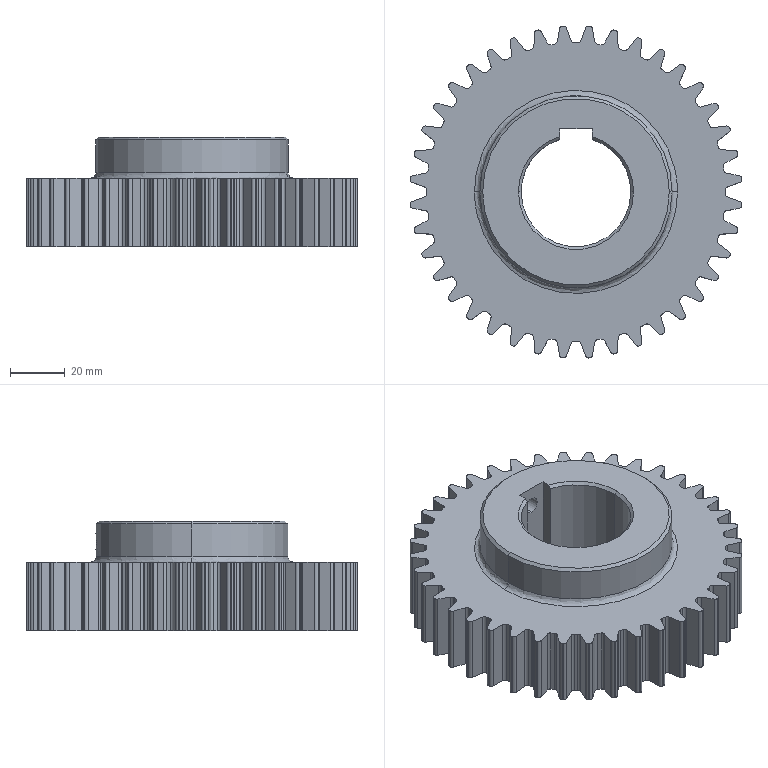Part | STEP file | Large pulley | 1 solid | 373 faces | box 120.932 x 120.932 x 40 mm | volume 261557 mm3 | cylinder 237 | plane 126 | cone 8 | spline 2 | commonest cylinder face diameters 2.34 x96 2.38 x94 121.28 x40 40 x3 6 x2 70 x2